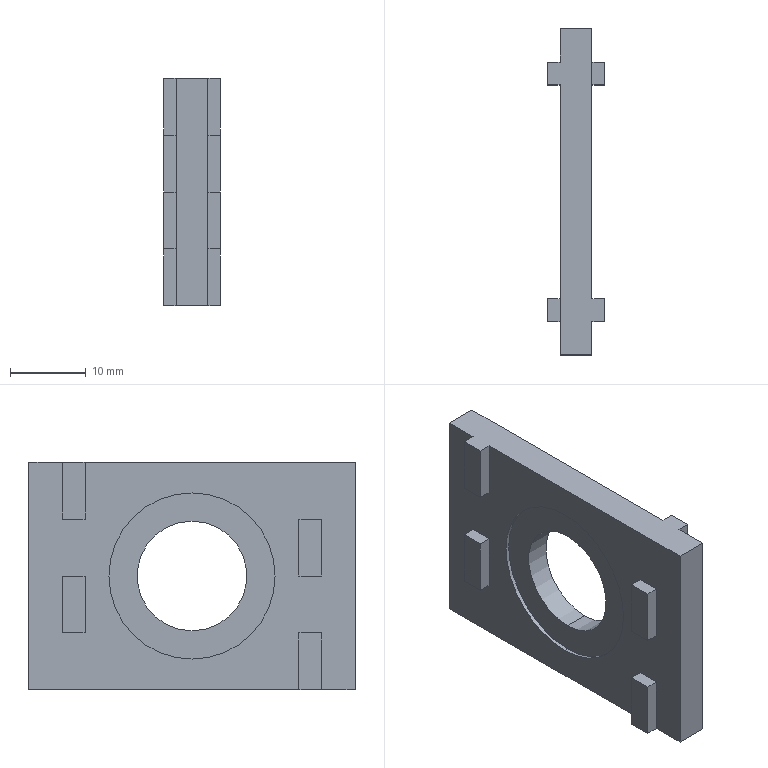Part | SolidWorks | features BaseBody 1 | 1 solid | 50 faces | box 7.5 x 43 x 30 mm | volume 4813 mm3 | plane 44 | cylinder 6 | commonest cylinder face diameters 21.9 x4 14.46 x2
STEP:
#1=CARTESIAN_POINT('',(-1.6,0.,7.23));
#2=VERTEX_POINT('',#1);
#3=CARTESIAN_POINT('',(-1.6,0.,-7.23));
#4=VERTEX_POINT('',#3);
#5=CARTESIAN_POINT('',(-1.6,0.,0.));
#6=DIRECTION('',(1.,0.,0.));
#7=DIRECTION('',(0.,0.,-1.));
#8=AXIS2_PLACEMENT_3D('',#5,#6,#7);
#9=CIRCLE('',#8,7.23);
#10=EDGE_CURVE('',#2,#4,#9,.T.);
#11=ORIENTED_EDGE('',*,*,#10,.F.);
#12=CARTESIAN_POINT('',(1.6,0.,7.23));
#13=VERTEX_POINT('',#12);
#14=CARTESIAN_POINT('',(2.1,0.,7.23));
#15=DIRECTION('',(1.,0.,0.));
#16=VECTOR('',#15,1000.);
#17=LINE('',#14,#16);
#18=EDGE_CURVE('',#2,#13,#17,.T.);
#19=ORIENTED_EDGE('',*,*,#18,.T.);
#20=CARTESIAN_POINT('',(1.6,0.,-7.23));
#21=VERTEX_POINT('',#20);
#22=CARTESIAN_POINT('',(1.6,0.,0.));
#23=DIRECTION('',(1.,0.,0.));
#24=DIRECTION('',(0.,0.,-1.));
#25=AXIS2_PLACEMENT_3D('',#22,#23,#24);
#26=CIRCLE('',#25,7.23);
#27=EDGE_CURVE('',#13,#21,#26,.T.);
#28=ORIENTED_EDGE('',*,*,#27,.T.);
#29=CARTESIAN_POINT('',(2.1,0.,-7.23));
#30=DIRECTION('',(1.,0.,0.));
#31=VECTOR('',#30,1000.);
#32=LINE('',#29,#31);
#33=EDGE_CURVE('',#4,#21,#32,.T.);
#34=ORIENTED_EDGE('',*,*,#33,.F.);
#35=EDGE_LOOP('',(#11,#19,#28,#34));
#36=FACE_OUTER_BOUND('',#35,.T.);
#37=CARTESIAN_POINT('',(2.1,0.,0.));
#38=DIRECTION('',(1.,0.,0.));
#39=DIRECTION('',(0.,0.,-1.));
#40=AXIS2_PLACEMENT_3D('',#37,#38,#39);
#41=CYLINDRICAL_SURFACE('',#40,7.23);
#42=ADVANCED_FACE('',(#36),#41,.F.);
#43=CARTESIAN_POINT('',(1.6,0.,10.95));
#44=VERTEX_POINT('',#43);
#45=CARTESIAN_POINT('',(1.6,0.,-10.95));
#46=VERTEX_POINT('',#45);
#47=CARTESIAN_POINT('',(1.6,0.,0.));
#48=DIRECTION('',(1.,0.,0.));
#49=DIRECTION('',(0.,0.,-1.));
#50=AXIS2_PLACEMENT_3D('',#47,#48,#49);
#51=CIRCLE('',#50,10.95);
#52=EDGE_CURVE('',#44,#46,#51,.T.);
#53=ORIENTED_EDGE('',*,*,#52,.F.);
#54=CARTESIAN_POINT('',(2.1,0.,10.95));
#55=VERTEX_POINT('',#54);
#56=CARTESIAN_POINT('',(2.1,0.,10.95));
#57=DIRECTION('',(1.,0.,0.));
#58=VECTOR('',#57,1000.);
#59=LINE('',#56,#58);
#60=EDGE_CURVE('',#44,#55,#59,.T.);
#61=ORIENTED_EDGE('',*,*,#60,.T.);
#62=CARTESIAN_POINT('',(2.1,0.,-10.95));
#63=VERTEX_POINT('',#62);
#64=CARTESIAN_POINT('',(2.1,0.,0.));
#65=DIRECTION('',(1.,0.,0.));
#66=DIRECTION('',(0.,0.,-1.));
#67=AXIS2_PLACEMENT_3D('',#64,#65,#66);
#68=CIRCLE('',#67,10.95);
#69=EDGE_CURVE('',#55,#63,#68,.T.);
#70=ORIENTED_EDGE('',*,*,#69,.T.);
#71=CARTESIAN_POINT('',(2.1,0.,-10.95));
#72=DIRECTION('',(1.,0.,0.));
#73=VECTOR('',#72,1000.);
#74=LINE('',#71,#73);
#75=EDGE_CURVE('',#46,#63,#74,.T.);
#76=ORIENTED_EDGE('',*,*,#75,.F.);
#77=EDGE_LOOP('',(#53,#61,#70,#76));
#78=FACE_OUTER_BOUND('',#77,.T.);
#79=CARTESIAN_POINT('',(2.1,0.,0.));
#80=DIRECTION('',(1.,0.,0.));
#81=DIRECTION('',(0.,0.,-1.));
#82=AXIS2_PLACEMENT_3D('',#79,#80,#81);
#83=CYLINDRICAL_SURFACE('',#82,10.95);
#84=ADVANCED_FACE('',(#78),#83,.F.);
#85=CARTESIAN_POINT('',(-2.1,0.,10.95));
#86=VERTEX_POINT('',#85);
#87=CARTESIAN_POINT('',(-2.1,0.,-10.95));
#88=VERTEX_POINT('',#87);
#89=CARTESIAN_POINT('',(-2.1,0.,0.));
#90=DIRECTION('',(1.,0.,0.));
#91=DIRECTION('',(0.,0.,-1.));
#92=AXIS2_PLACEMENT_3D('',#89,#90,#91);
#93=CIRCLE('',#92,10.95);
#94=EDGE_CURVE('',#86,#88,#93,.T.);
#95=ORIENTED_EDGE('',*,*,#94,.F.);
#96=CARTESIAN_POINT('',(-1.6,0.,10.95));
#97=VERTEX_POINT('',#96);
#98=CARTESIAN_POINT('',(2.1,0.,10.95));
#99=DIRECTION('',(1.,0.,0.));
#100=VECTOR('',#99,1000.);
#101=LINE('',#98,#100);
#102=EDGE_CURVE('',#86,#97,#101,.T.);
#103=ORIENTED_EDGE('',*,*,#102,.T.);
#104=CARTESIAN_POINT('',(-1.6,0.,-10.95));
#105=VERTEX_POINT('',#104);
#106=CARTESIAN_POINT('',(-1.6,0.,0.));
#107=DIRECTION('',(1.,0.,0.));
#108=DIRECTION('',(0.,0.,-1.));
#109=AXIS2_PLACEMENT_3D('',#106,#107,#108);
#110=CIRCLE('',#109,10.95);
#111=EDGE_CURVE('',#97,#105,#110,.T.);
#112=ORIENTED_EDGE('',*,*,#111,.T.);
#113=CARTESIAN_POINT('',(2.1,0.,-10.95));
#114=DIRECTION('',(1.,0.,0.));
#115=VECTOR('',#114,1000.);
#116=LINE('',#113,#115);
#117=EDGE_CURVE('',#88,#105,#116,.T.);
#118=ORIENTED_EDGE('',*,*,#117,.F.);
#119=EDGE_LOOP('',(#95,#103,#112,#118));
#120=FACE_OUTER_BOUND('',#119,.T.);
#121=CARTESIAN_POINT('',(2.1,0.,0.));
#122=DIRECTION('',(1.,0.,0.));
#123=DIRECTION('',(0.,0.,-1.));
#124=AXIS2_PLACEMENT_3D('',#121,#122,#123);
#125=CYLINDRICAL_SURFACE('',#124,10.95);
#126=ADVANCED_FACE('',(#120),#125,.F.);
#127=CARTESIAN_POINT('',(-3.75,-14.1,-7.5));
#128=VERTEX_POINT('',#127);
#129=CARTESIAN_POINT('',(-3.75,-14.1,-15.));
#130=VERTEX_POINT('',#129);
#131=CARTESIAN_POINT('',(-3.75,-14.1,-7.5));
#132=DIRECTION('',(0.,0.,-1.));
#133=VECTOR('',#132,1000.);
#134=LINE('',#131,#133);
#135=EDGE_CURVE('',#128,#130,#134,.T.);
#136=ORIENTED_EDGE('',*,*,#135,.F.);
#137=CARTESIAN_POINT('',(-2.1,-14.1,-7.5));
#138=VERTEX_POINT('',#137);
#139=CARTESIAN_POINT('',(-3.75,-14.1,-7.5));
#140=DIRECTION('',(1.,0.,0.));
#141=VECTOR('',#140,1000.);
#142=LINE('',#139,#141);
#143=EDGE_CURVE('',#128,#138,#142,.T.);
#144=ORIENTED_EDGE('',*,*,#143,.T.);
#145=CARTESIAN_POINT('',(-2.1,-14.1,-15.));
#146=VERTEX_POINT('',#145);
#147=CARTESIAN_POINT('',(-2.1,-14.1,-7.5));
#148=DIRECTION('',(0.,0.,-1.));
#149=VECTOR('',#148,1000.);
#150=LINE('',#147,#149);
#151=EDGE_CURVE('',#138,#146,#150,.T.);
#152=ORIENTED_EDGE('',*,*,#151,.T.);
#153=CARTESIAN_POINT('',(-2.1,-14.1,-15.));
#154=DIRECTION('',(-1.,0.,0.));
#155=VECTOR('',#154,1000.);
#156=LINE('',#153,#155);
#157=EDGE_CURVE('',#146,#130,#156,.T.);
#158=ORIENTED_EDGE('',*,*,#157,.T.);
#159=EDGE_LOOP('',(#136,#144,#152,#158));
#160=FACE_OUTER_BOUND('',#159,.T.);
#161=CARTESIAN_POINT('',(-2.1,-14.1,15.));
#162=DIRECTION('',(0.,-1.,0.));
#163=DIRECTION('',(0.,0.,-1.));
#164=AXIS2_PLACEMENT_3D('',#161,#162,#163);
#165=PLANE('',#164);
#166=ADVANCED_FACE('',(#160),#165,.F.);
#167=CARTESIAN_POINT('',(-3.75,-17.1,-7.5));
#168=VERTEX_POINT('',#167);
#169=CARTESIAN_POINT('',(-3.75,-17.1,-15.));
#170=VERTEX_POINT('',#169);
#171=CARTESIAN_POINT('',(-3.75,-17.1,-7.5));
#172=DIRECTION('',(0.,0.,-1.));
#173=VECTOR('',#172,1000.);
#174=LINE('',#171,#173);
#175=EDGE_CURVE('',#168,#170,#174,.T.);
#176=ORIENTED_EDGE('',*,*,#175,.F.);
#177=CARTESIAN_POINT('',(-3.75,-17.1,-7.5));
#178=DIRECTION('',(0.,1.,0.));
#179=VECTOR('',#178,1000.);
#180=LINE('',#177,#179);
#181=EDGE_CURVE('',#168,#128,#180,.T.);
#182=ORIENTED_EDGE('',*,*,#181,.T.);
#183=ORIENTED_EDGE('',*,*,#135,.T.);
#184=CARTESIAN_POINT('',(-3.75,-14.1,-15.));
#185=DIRECTION('',(0.,-1.,0.));
#186=VECTOR('',#185,1000.);
#187=LINE('',#184,#186);
#188=EDGE_CURVE('',#130,#170,#187,.T.);
#189=ORIENTED_EDGE('',*,*,#188,.T.);
#190=EDGE_LOOP('',(#176,#182,#183,#189));
#191=FACE_OUTER_BOUND('',#190,.T.);
#192=CARTESIAN_POINT('',(-3.75,-14.1,15.));
#193=DIRECTION('',(1.,0.,0.));
#194=DIRECTION('',(0.,0.,-1.));
#195=AXIS2_PLACEMENT_3D('',#192,#193,#194);
#196=PLANE('',#195);
#197=ADVANCED_FACE('',(#191),#196,.F.);
#198=ORIENTED_EDGE('',*,*,#181,.F.);
#199=CARTESIAN_POINT('',(-2.1,-17.1,-7.5));
#200=VERTEX_POINT('',#199);
#201=CARTESIAN_POINT('',(-2.1,-17.1,-7.5));
#202=DIRECTION('',(-1.,0.,0.));
#203=VECTOR('',#202,1000.);
#204=LINE('',#201,#203);
#205=EDGE_CURVE('',#200,#168,#204,.T.);
#206=ORIENTED_EDGE('',*,*,#205,.F.);
#207=CARTESIAN_POINT('',(-2.1,-17.1,-7.5));
#208=DIRECTION('',(0.,1.,0.));
#209=VECTOR('',#208,1000.);
#210=LINE('',#207,#209);
#211=EDGE_CURVE('',#200,#138,#210,.T.);
#212=ORIENTED_EDGE('',*,*,#211,.T.);
#213=ORIENTED_EDGE('',*,*,#143,.F.);
#214=EDGE_LOOP('',(#198,#206,#212,#213));
#215=FACE_OUTER_BOUND('',#214,.T.);
#216=CARTESIAN_POINT('',(-2.1,-21.5,-7.5));
#217=DIRECTION('',(0.,0.,-1.));
#218=DIRECTION('',(-1.,0.,0.));
#219=AXIS2_PLACEMENT_3D('',#216,#217,#218);
#220=PLANE('',#219);
#221=ADVANCED_FACE('',(#215),#220,.F.);
#222=CARTESIAN_POINT('',(-2.1,0.,0.));
#223=DIRECTION('',(1.,0.,0.));
#224=DIRECTION('',(0.,0.,-1.));
#225=AXIS2_PLACEMENT_3D('',#222,#223,#224);
#226=CIRCLE('',#225,10.95);
#227=EDGE_CURVE('',#88,#86,#226,.T.);
#228=ORIENTED_EDGE('',*,*,#227,.T.);
#229=ORIENTED_EDGE('',*,*,#94,.T.);
#230=EDGE_LOOP('',(#228,#229));
#231=FACE_BOUND('',#230,.T.);
#232=CARTESIAN_POINT('',(-2.1,-14.1,7.5));
#233=VERTEX_POINT('',#232);
#234=CARTESIAN_POINT('',(-2.1,-14.1,0.));
#235=VERTEX_POINT('',#234);
#236=CARTESIAN_POINT('',(-2.1,-14.1,7.5));
#237=DIRECTION('',(0.,0.,-1.));
#238=VECTOR('',#237,1000.);
#239=LINE('',#236,#238);
#240=EDGE_CURVE('',#233,#235,#239,.T.);
#241=ORIENTED_EDGE('',*,*,#240,.F.);
#242=CARTESIAN_POINT('',(-2.1,-17.1,7.5));
#243=VERTEX_POINT('',#242);
#244=CARTESIAN_POINT('',(-2.1,-17.1,7.5));
#245=DIRECTION('',(0.,1.,0.));
#246=VECTOR('',#245,1000.);
#247=LINE('',#244,#246);
#248=EDGE_CURVE('',#243,#233,#247,.T.);
#249=ORIENTED_EDGE('',*,*,#248,.F.);
#250=CARTESIAN_POINT('',(-2.1,-17.1,0.));
#251=VERTEX_POINT('',#250);
#252=CARTESIAN_POINT('',(-2.1,-17.1,7.5));
#253=DIRECTION('',(0.,0.,-1.));
#254=VECTOR('',#253,1000.);
#255=LINE('',#252,#254);
#256=EDGE_CURVE('',#243,#251,#255,.T.);
#257=ORIENTED_EDGE('',*,*,#256,.T.);
#258=CARTESIAN_POINT('',(-2.1,-17.1,0.));
#259=DIRECTION('',(0.,1.,0.));
#260=VECTOR('',#259,1000.);
#261=LINE('',#258,#260);
#262=EDGE_CURVE('',#251,#235,#261,.T.);
#263=ORIENTED_EDGE('',*,*,#262,.T.);
#264=EDGE_LOOP('',(#241,#249,#257,#263));
#265=FACE_BOUND('',#264,.T.);
#266=ORIENTED_EDGE('',*,*,#151,.F.);
#267=ORIENTED_EDGE('',*,*,#211,.F.);
#268=CARTESIAN_POINT('',(-2.1,-17.1,-15.));
#269=VERTEX_POINT('',#268);
#270=CARTESIAN_POINT('',(-2.1,-17.1,-7.5));
#271=DIRECTION('',(0.,0.,-1.));
#272=VECTOR('',#271,1000.);
#273=LINE('',#270,#272);
#274=EDGE_CURVE('',#200,#269,#273,.T.);
#275=ORIENTED_EDGE('',*,*,#274,.T.);
#276=CARTESIAN_POINT('',(-2.1,-21.5,-15.));
#277=VERTEX_POINT('',#276);
#278=CARTESIAN_POINT('',(-2.1,-17.1,-15.));
#279=DIRECTION('',(0.,-1.,0.));
#280=VECTOR('',#279,1000.);
#281=LINE('',#278,#280);
#282=EDGE_CURVE('',#269,#277,#281,.T.);
#283=ORIENTED_EDGE('',*,*,#282,.T.);
#284=CARTESIAN_POINT('',(-2.1,-21.5,15.));
#285=VERTEX_POINT('',#284);
#286=CARTESIAN_POINT('',(-2.1,-21.5,15.));
#287=DIRECTION('',(0.,0.,-1.));
#288=VECTOR('',#287,1000.);
#289=LINE('',#286,#288);
#290=EDGE_CURVE('',#285,#277,#289,.T.);
#291=ORIENTED_EDGE('',*,*,#290,.F.);
#292=CARTESIAN_POINT('',(-2.1,14.1,15.));
#293=VERTEX_POINT('',#292);
#294=CARTESIAN_POINT('',(-2.1,14.1,15.));
#295=DIRECTION('',(0.,-1.,0.));
#296=VECTOR('',#295,1000.);
#297=LINE('',#294,#296);
#298=EDGE_CURVE('',#293,#285,#297,.T.);
#299=ORIENTED_EDGE('',*,*,#298,.F.);
#300=CARTESIAN_POINT('',(-2.1,14.1,7.5));
#301=VERTEX_POINT('',#300);
#302=CARTESIAN_POINT('',(-2.1,14.1,15.));
#303=DIRECTION('',(0.,0.,-1.));
#304=VECTOR('',#303,1000.);
#305=LINE('',#302,#304);
#306=EDGE_CURVE('',#293,#301,#305,.T.);
#307=ORIENTED_EDGE('',*,*,#306,.T.);
#308=CARTESIAN_POINT('',(-2.1,17.1,7.5));
#309=VERTEX_POINT('',#308);
#310=CARTESIAN_POINT('',(-2.1,17.1,7.5));
#311=DIRECTION('',(0.,-1.,0.));
#312=VECTOR('',#311,1000.);
#313=LINE('',#310,#312);
#314=EDGE_CURVE('',#309,#301,#313,.T.);
#315=ORIENTED_EDGE('',*,*,#314,.F.);
#316=CARTESIAN_POINT('',(-2.1,17.1,15.));
#317=VERTEX_POINT('',#316);
#318=CARTESIAN_POINT('',(-2.1,17.1,15.));
#319=DIRECTION('',(0.,0.,-1.));
#320=VECTOR('',#319,1000.);
#321=LINE('',#318,#320);
#322=EDGE_CURVE('',#317,#309,#321,.T.);
#323=ORIENTED_EDGE('',*,*,#322,.F.);
#324=CARTESIAN_POINT('',(-2.1,21.5,15.));
#325=VERTEX_POINT('',#324);
#326=CARTESIAN_POINT('',(-2.1,21.5,15.));
#327=DIRECTION('',(0.,-1.,0.));
#328=VECTOR('',#327,1000.);
#329=LINE('',#326,#328);
#330=EDGE_CURVE('',#325,#317,#329,.T.);
#331=ORIENTED_EDGE('',*,*,#330,.F.);
#332=CARTESIAN_POINT('',(-2.1,21.5,-15.));
#333=VERTEX_POINT('',#332);
#334=CARTESIAN_POINT('',(-2.1,21.5,15.));
#335=DIRECTION('',(0.,0.,-1.));
#336=VECTOR('',#335,1000.);
#337=LINE('',#334,#336);
#338=EDGE_CURVE('',#325,#333,#337,.T.);
#339=ORIENTED_EDGE('',*,*,#338,.T.);
#340=CARTESIAN_POINT('',(-2.1,21.5,-15.));
#341=DIRECTION('',(0.,-1.,0.));
#342=VECTOR('',#341,1000.);
#343=LINE('',#340,#342);
#344=EDGE_CURVE('',#333,#146,#343,.T.);
#345=ORIENTED_EDGE('',*,*,#344,.T.);
#346=EDGE_LOOP('',(#266,#267,#275,#283,#291,#299,#307,#315,#323,#331,#339,#345));
#347=FACE_OUTER_BOUND('',#346,.T.);
#348=CARTESIAN_POINT('',(-2.1,17.1,0.));
#349=VERTEX_POINT('',#348);
#350=CARTESIAN_POINT('',(-2.1,14.1,0.));
#351=VERTEX_POINT('',#350);
#352=CARTESIAN_POINT('',(-2.1,17.1,0.));
#353=DIRECTION('',(0.,-1.,0.));
#354=VECTOR('',#353,1000.);
#355=LINE('',#352,#354);
#356=EDGE_CURVE('',#349,#351,#355,.T.);
#357=ORIENTED_EDGE('',*,*,#356,.T.);
#358=CARTESIAN_POINT('',(-2.1,14.1,-7.5));
#359=VERTEX_POINT('',#358);
#360=CARTESIAN_POINT('',(-2.1,14.1,0.));
#361=DIRECTION('',(0.,0.,-1.));
#362=VECTOR('',#361,1000.);
#363=LINE('',#360,#362);
#364=EDGE_CURVE('',#351,#359,#363,.T.);
#365=ORIENTED_EDGE('',*,*,#364,.T.);
#366=CARTESIAN_POINT('',(-2.1,17.1,-7.5));
#367=VERTEX_POINT('',#366);
#368=CARTESIAN_POINT('',(-2.1,17.1,-7.5));
#369=DIRECTION('',(0.,-1.,0.));
#370=VECTOR('',#369,1000.);
#371=LINE('',#368,#370);
#372=EDGE_CURVE('',#367,#359,#371,.T.);
#373=ORIENTED_EDGE('',*,*,#372,.F.);
#374=CARTESIAN_POINT('',(-2.1,17.1,0.));
#375=DIRECTION('',(0.,0.,-1.));
#376=VECTOR('',#375,1000.);
#377=LINE('',#374,#376);
#378=EDGE_CURVE('',#349,#367,#377,.T.);
#379=ORIENTED_EDGE('',*,*,#378,.F.);
#380=EDGE_LOOP('',(#357,#365,#373,#379));
#381=FACE_BOUND('',#380,.T.);
#382=CARTESIAN_POINT('',(-2.1,21.5,15.));
#383=DIRECTION('',(1.,0.,0.));
#384=DIRECTION('',(0.,0.,-1.));
#385=AXIS2_PLACEMENT_3D('',#382,#383,#384);
#386=PLANE('',#385);
#387=ADVANCED_FACE('',(#231,#265,#347,#381),#386,.F.);
#388=ORIENTED_EDGE('',*,*,#157,.F.);
#389=ORIENTED_EDGE('',*,*,#344,.F.);
#390=CARTESIAN_POINT('',(2.1,21.5,-15.));
#391=VERTEX_POINT('',#390);
#392=CARTESIAN_POINT('',(2.1,21.5,-15.));
#393=DIRECTION('',(-1.,0.,0.));
#394=VECTOR('',#393,1000.);
#395=LINE('',#392,#394);
#396=EDGE_CURVE('',#391,#333,#395,.T.);
#397=ORIENTED_EDGE('',*,*,#396,.F.);
#398=CARTESIAN_POINT('',(2.1,17.1,-15.));
#399=VERTEX_POINT('',#398);
#400=CARTESIAN_POINT('',(2.1,17.1,-15.));
#401=DIRECTION('',(0.,1.,0.));
#402=VECTOR('',#401,1000.);
#403=LINE('',#400,#402);
#404=EDGE_CURVE('',#399,#391,#403,.T.);
#405=ORIENTED_EDGE('',*,*,#404,.F.);
#406=CARTESIAN_POINT('',(3.75,17.1,-15.));
#407=VERTEX_POINT('',#406);
#408=CARTESIAN_POINT('',(3.75,17.1,-15.));
#409=DIRECTION('',(-1.,0.,0.));
#410=VECTOR('',#409,1000.);
#411=LINE('',#408,#410);
#412=EDGE_CURVE('',#407,#399,#411,.T.);
#413=ORIENTED_EDGE('',*,*,#412,.F.);
#414=CARTESIAN_POINT('',(3.75,14.1,-15.));
#415=VERTEX_POINT('',#414);
#416=CARTESIAN_POINT('',(3.75,14.1,-15.));
#417=DIRECTION('',(0.,1.,0.));
#418=VECTOR('',#417,1000.);
#419=LINE('',#416,#418);
#420=EDGE_CURVE('',#415,#407,#419,.T.);
#421=ORIENTED_EDGE('',*,*,#420,.F.);
#422=CARTESIAN_POINT('',(2.1,14.1,-15.));
#423=VERTEX_POINT('',#422);
#424=CARTESIAN_POINT('',(2.1,14.1,-15.));
#425=DIRECTION('',(1.,0.,0.));
#426=VECTOR('',#425,1000.);
#427=LINE('',#424,#426);
#428=EDGE_CURVE('',#423,#415,#427,.T.);
#429=ORIENTED_EDGE('',*,*,#428,.F.);
#430=CARTESIAN_POINT('',(2.1,-21.5,-15.));
#431=VERTEX_POINT('',#430);
#432=CARTESIAN_POINT('',(2.1,-21.5,-15.));
#433=DIRECTION('',(0.,1.,0.));
#434=VECTOR('',#433,1000.);
#435=LINE('',#432,#434);
#436=EDGE_CURVE('',#431,#423,#435,.T.);
#437=ORIENTED_EDGE('',*,*,#436,.F.);
#438=CARTESIAN_POINT('',(-2.1,-21.5,-15.));
#439=DIRECTION('',(1.,0.,0.));
#440=VECTOR('',#439,1000.);
#441=LINE('',#438,#440);
#442=EDGE_CURVE('',#277,#431,#441,.T.);
#443=ORIENTED_EDGE('',*,*,#442,.F.);
#444=ORIENTED_EDGE('',*,*,#282,.F.);
#445=CARTESIAN_POINT('',(-3.75,-17.1,-15.));
#446=DIRECTION('',(1.,0.,0.));
#447=VECTOR('',#446,1000.);
#448=LINE('',#445,#447);
#449=EDGE_CURVE('',#170,#269,#448,.T.);
#450=ORIENTED_EDGE('',*,*,#449,.F.);
#451=ORIENTED_EDGE('',*,*,#188,.F.);
#452=EDGE_LOOP('',(#388,#389,#397,#405,#413,#421,#429,#437,#443,#444,#450,#451));
#453=FACE_OUTER_BOUND('',#452,.T.);
#454=CARTESIAN_POINT('',(0.,0.,-15.));
#455=DIRECTION('',(0.,0.,1.));
#456=DIRECTION('',(1.,0.,0.));
#457=AXIS2_PLACEMENT_3D('',#454,#455,#456);
#458=PLANE('',#457);
#459=ADVANCED_FACE('',(#453),#458,.F.);
#460=ORIENTED_EDGE('',*,*,#274,.F.);
#461=ORIENTED_EDGE('',*,*,#205,.T.);
#462=ORIENTED_EDGE('',*,*,#175,.T.);
#463=ORIENTED_EDGE('',*,*,#449,.T.);
#464=EDGE_LOOP('',(#460,#461,#462,#463));
#465=FACE_OUTER_BOUND('',#464,.T.);
#466=CARTESIAN_POINT('',(-3.75,-17.1,15.));
#467=DIRECTION('',(0.,1.,0.));
#468=DIRECTION('',(0.,0.,1.));
#469=AXIS2_PLACEMENT_3D('',#466,#467,#468);
#470=PLANE('',#469);
#471=ADVANCED_FACE('',(#465),#470,.F.);
#472=ORIENTED_EDGE('',*,*,#102,.F.);
#473=ORIENTED_EDGE('',*,*,#227,.F.);
#474=ORIENTED_EDGE('',*,*,#117,.T.);
#475=CARTESIAN_POINT('',(-1.6,0.,0.));
#476=DIRECTION('',(1.,0.,0.));
#477=DIRECTION('',(0.,0.,-1.));
#478=AXIS2_PLACEMENT_3D('',#475,#476,#477);
#479=CIRCLE('',#478,10.95);
#480=EDGE_CURVE('',#105,#97,#479,.T.);
#481=ORIENTED_EDGE('',*,*,#480,.T.);
#482=EDGE_LOOP('',(#472,#473,#474,#481));
#483=FACE_OUTER_BOUND('',#482,.T.);
#484=CARTESIAN_POINT('',(2.1,0.,0.));
#485=DIRECTION('',(1.,0.,0.));
#486=DIRECTION('',(0.,0.,-1.));
#487=AXIS2_PLACEMENT_3D('',#484,#485,#486);
#488=CYLINDRICAL_SURFACE('',#487,10.95);
#489=ADVANCED_FACE('',(#483),#488,.F.);
#490=CARTESIAN_POINT('',(-3.75,-14.1,7.5));
#491=VERTEX_POINT('',#490);
#492=CARTESIAN_POINT('',(-3.75,-14.1,0.));
#493=VERTEX_POINT('',#492);
#494=CARTESIAN_POINT('',(-3.75,-14.1,7.5));
#495=DIRECTION('',(0.,0.,-1.));
#496=VECTOR('',#495,1000.);
#497=LINE('',#494,#496);
#498=EDGE_CURVE('',#491,#493,#497,.T.);
#499=ORIENTED_EDGE('',*,*,#498,.F.);
#500=CARTESIAN_POINT('',(-3.75,-14.1,7.5));
#501=DIRECTION('',(1.,0.,0.));
#502=VECTOR('',#501,1000.);
#503=LINE('',#500,#502);
#504=EDGE_CURVE('',#491,#233,#503,.T.);
#505=ORIENTED_EDGE('',*,*,#504,.T.);
#506=ORIENTED_EDGE('',*,*,#240,.T.);
#507=CARTESIAN_POINT('',(-2.1,-14.1,0.));
#508=DIRECTION('',(-1.,0.,0.));
#509=VECTOR('',#508,1000.);
#510=LINE('',#507,#509);
#511=EDGE_CURVE('',#235,#493,#510,.T.);
#512=ORIENTED_EDGE('',*,*,#511,.T.);
#513=EDGE_LOOP('',(#499,#505,#506,#512));
#514=FACE_OUTER_BOUND('',#513,.T.);
#515=CARTESIAN_POINT('',(-2.1,-14.1,15.));
#516=DIRECTION('',(0.,-1.,0.));
#517=DIRECTION('',(0.,0.,-1.));
#518=AXIS2_PLACEMENT_3D('',#515,#516,#517);
#519=PLANE('',#518);
#520=ADVANCED_FACE('',(#514),#519,.F.);
#521=CARTESIAN_POINT('',(-3.75,-17.1,7.5));
#522=VERTEX_POINT('',#521);
#523=CARTESIAN_POINT('',(-3.75,-17.1,7.5));
#524=DIRECTION('',(0.,1.,0.));
#525=VECTOR('',#524,1000.);
#526=LINE('',#523,#525);
#527=EDGE_CURVE('',#522,#491,#526,.T.);
#528=ORIENTED_EDGE('',*,*,#527,.F.);
#529=CARTESIAN_POINT('',(-2.1,-17.1,7.5));
#530=DIRECTION('',(-1.,0.,0.));
#531=VECTOR('',#530,1000.);
#532=LINE('',#529,#531);
#533=EDGE_CURVE('',#243,#522,#532,.T.);
#534=ORIENTED_EDGE('',*,*,#533,.F.);
#535=ORIENTED_EDGE('',*,*,#248,.T.);
#536=ORIENTED_EDGE('',*,*,#504,.F.);
#537=EDGE_LOOP('',(#528,#534,#535,#536));
#538=FACE_OUTER_BOUND('',#537,.T.);
#539=CARTESIAN_POINT('',(-2.1,-21.5,7.5));
#540=DIRECTION('',(0.,0.,-1.));
#541=DIRECTION('',(-1.,0.,0.));
#542=AXIS2_PLACEMENT_3D('',#539,#540,#541);
#543=PLANE('',#542);
#544=ADVANCED_FACE('',(#538),#543,.F.);
#545=ORIENTED_EDGE('',*,*,#256,.F.);
#546=ORIENTED_EDGE('',*,*,#533,.T.);
#547=CARTESIAN_POINT('',(-3.75,-17.1,0.));
#548=VERTEX_POINT('',#547);
#549=CARTESIAN_POINT('',(-3.75,-17.1,7.5));
#550=DIRECTION('',(0.,0.,-1.));
#551=VECTOR('',#550,1000.);
#552=LINE('',#549,#551);
#553=EDGE_CURVE('',#522,#548,#552,.T.);
#554=ORIENTED_EDGE('',*,*,#553,.T.);
#555=CARTESIAN_POINT('',(-3.75,-17.1,0.));
#556=DIRECTION('',(1.,0.,0.));
#557=VECTOR('',#556,1000.);
#558=LINE('',#555,#557);
#559=EDGE_CURVE('',#548,#251,#558,.T.);
#560=ORIENTED_EDGE('',*,*,#559,.T.);
#561=EDGE_LOOP('',(#545,#546,#554,#560));
#562=FACE_OUTER_BOUND('',#561,.T.);
#563=CARTESIAN_POINT('',(-3.75,-17.1,15.));
#564=DIRECTION('',(0.,1.,0.));
#565=DIRECTION('',(0.,0.,1.));
#566=AXIS2_PLACEMENT_3D('',#563,#564,#565);
#567=PLANE('',#566);
#568=ADVANCED_FACE('',(#562),#567,.F.);
#569=ORIENTED_EDGE('',*,*,#262,.F.);
#570=ORIENTED_EDGE('',*,*,#559,.F.);
#571=CARTESIAN_POINT('',(-3.75,-17.1,0.));
#572=DIRECTION('',(0.,1.,0.));
#573=VECTOR('',#572,1000.);
#574=LINE('',#571,#573);
#575=EDGE_CURVE('',#548,#493,#574,.T.);
#576=ORIENTED_EDGE('',*,*,#575,.T.);
#577=ORIENTED_EDGE('',*,*,#511,.F.);
#578=EDGE_LOOP('',(#569,#570,#576,#577));
#579=FACE_OUTER_BOUND('',#578,.T.);
#580=CARTESIAN_POINT('',(-3.75,-21.5,0.));
#581=DIRECTION('',(0.,0.,1.));
#582=DIRECTION('',(1.,0.,0.));
#583=AXIS2_PLACEMENT_3D('',#580,#581,#582);
#584=PLANE('',#583);
#585=ADVANCED_FACE('',(#579),#584,.F.);
#586=ORIENTED_EDGE('',*,*,#442,.T.);
#587=CARTESIAN_POINT('',(2.1,-21.5,15.));
#588=VERTEX_POINT('',#587);
#589=CARTESIAN_POINT('',(2.1,-21.5,15.));
#590=DIRECTION('',(0.,0.,-1.));
#591=VECTOR('',#590,1000.);
#592=LINE('',#589,#591);
#593=EDGE_CURVE('',#588,#431,#592,.T.);
#594=ORIENTED_EDGE('',*,*,#593,.F.);
#595=CARTESIAN_POINT('',(-2.1,-21.5,15.));
#596=DIRECTION('',(1.,0.,0.));
#597=VECTOR('',#596,1000.);
#598=LINE('',#595,#597);
#599=EDGE_CURVE('',#285,#588,#598,.T.);
#600=ORIENTED_EDGE('',*,*,#599,.F.);
#601=ORIENTED_EDGE('',*,*,#290,.T.);
#602=EDGE_LOOP('',(#586,#594,#600,#601));
#603=FACE_OUTER_BOUND('',#602,.T.);
#604=CARTESIAN_POINT('',(-2.1,-21.5,15.));
#605=DIRECTION('',(0.,1.,0.));
#606=DIRECTION('',(0.,0.,1.));
#607=AXIS2_PLACEMENT_3D('',#604,#605,#606);
#608=PLANE('',#607);
#609=ADVANCED_FACE('',(#603),#608,.F.);
#610=ORIENTED_EDGE('',*,*,#298,.T.);
#611=ORIENTED_EDGE('',*,*,#599,.T.);
#612=CARTESIAN_POINT('',(2.1,-17.1,15.));
#613=VERTEX_POINT('',#612);
#614=CARTESIAN_POINT('',(2.1,-21.5,15.));
#615=DIRECTION('',(0.,1.,0.));
#616=VECTOR('',#615,1000.);
#617=LINE('',#614,#616);
#618=EDGE_CURVE('',#588,#613,#617,.T.);
#619=ORIENTED_EDGE('',*,*,#618,.T.);
#620=CARTESIAN_POINT('',(3.75,-17.1,15.));
#621=VERTEX_POINT('',#620);
#622=CARTESIAN_POINT('',(2.1,-17.1,15.));
#623=DIRECTION('',(1.,0.,0.));
#624=VECTOR('',#623,1000.);
#625=LINE('',#622,#624);
#626=EDGE_CURVE('',#613,#621,#625,.T.);
#627=ORIENTED_EDGE('',*,*,#626,.T.);
#628=CARTESIAN_POINT('',(3.75,-14.1,15.));
#629=VERTEX_POINT('',#628);
#630=CARTESIAN_POINT('',(3.75,-17.1,15.));
#631=DIRECTION('',(0.,1.,0.));
#632=VECTOR('',#631,1000.);
#633=LINE('',#630,#632);
#634=EDGE_CURVE('',#621,#629,#633,.T.);
#635=ORIENTED_EDGE('',*,*,#634,.T.);
#636=CARTESIAN_POINT('',(2.1,-14.1,15.));
#637=VERTEX_POINT('',#636);
#638=CARTESIAN_POINT('',(3.75,-14.1,15.));
#639=DIRECTION('',(-1.,0.,0.));
#640=VECTOR('',#639,1000.);
#641=LINE('',#638,#640);
#642=EDGE_CURVE('',#629,#637,#641,.T.);
#643=ORIENTED_EDGE('',*,*,#642,.T.);
#644=CARTESIAN_POINT('',(2.1,21.5,15.));
#645=VERTEX_POINT('',#644);
#646=CARTESIAN_POINT('',(2.1,-14.1,15.));
#647=DIRECTION('',(0.,1.,0.));
#648=VECTOR('',#647,1000.);
#649=LINE('',#646,#648);
#650=EDGE_CURVE('',#637,#645,#649,.T.);
#651=ORIENTED_EDGE('',*,*,#650,.T.);
#652=CARTESIAN_POINT('',(2.1,21.5,15.));
#653=DIRECTION('',(-1.,0.,0.));
#654=VECTOR('',#653,1000.);
#655=LINE('',#652,#654);
#656=EDGE_CURVE('',#645,#325,#655,.T.);
#657=ORIENTED_EDGE('',*,*,#656,.T.);
#658=ORIENTED_EDGE('',*,*,#330,.T.);
#659=CARTESIAN_POINT('',(-3.75,17.1,15.));
#660=VERTEX_POINT('',#659);
#661=CARTESIAN_POINT('',(-2.1,17.1,15.));
#662=DIRECTION('',(-1.,0.,0.));
#663=VECTOR('',#662,1000.);
#664=LINE('',#661,#663);
#665=EDGE_CURVE('',#317,#660,#664,.T.);
#666=ORIENTED_EDGE('',*,*,#665,.T.);
#667=CARTESIAN_POINT('',(-3.75,14.1,15.));
#668=VERTEX_POINT('',#667);
#669=CARTESIAN_POINT('',(-3.75,17.1,15.));
#670=DIRECTION('',(0.,-1.,0.));
#671=VECTOR('',#670,1000.);
#672=LINE('',#669,#671);
#673=EDGE_CURVE('',#660,#668,#672,.T.);
#674=ORIENTED_EDGE('',*,*,#673,.T.);
#675=CARTESIAN_POINT('',(-3.75,14.1,15.));
#676=DIRECTION('',(1.,0.,0.));
#677=VECTOR('',#676,1000.);
#678=LINE('',#675,#677);
#679=EDGE_CURVE('',#668,#293,#678,.T.);
#680=ORIENTED_EDGE('',*,*,#679,.T.);
#681=EDGE_LOOP('',(#610,#611,#619,#627,#635,#643,#651,#657,#658,#666,#674,#680));
#682=FACE_OUTER_BOUND('',#681,.T.);
#683=CARTESIAN_POINT('',(0.,0.,15.));
#684=DIRECTION('',(0.,0.,1.));
#685=DIRECTION('',(1.,0.,0.));
#686=AXIS2_PLACEMENT_3D('',#683,#684,#685);
#687=PLANE('',#686);
#688=ADVANCED_FACE('',(#682),#687,.T.);
#689=CARTESIAN_POINT('',(-3.75,14.1,7.5));
#690=VERTEX_POINT('',#689);
#691=CARTESIAN_POINT('',(-2.1,14.1,7.5));
#692=DIRECTION('',(-1.,0.,0.));
#693=VECTOR('',#692,1000.);
#694=LINE('',#691,#693);
#695=EDGE_CURVE('',#301,#690,#694,.T.);
#696=ORIENTED_EDGE('',*,*,#695,.F.);
#697=ORIENTED_EDGE('',*,*,#306,.F.);
#698=ORIENTED_EDGE('',*,*,#679,.F.);
#699=CARTESIAN_POINT('',(-3.75,14.1,15.));
#700=DIRECTION('',(0.,0.,-1.));
#701=VECTOR('',#700,1000.);
#702=LINE('',#699,#701);
#703=EDGE_CURVE('',#668,#690,#702,.T.);
#704=ORIENTED_EDGE('',*,*,#703,.T.);
#705=EDGE_LOOP('',(#696,#697,#698,#704));
#706=FACE_OUTER_BOUND('',#705,.T.);
#707=CARTESIAN_POINT('',(-3.75,14.1,15.));
#708=DIRECTION('',(0.,1.,0.));
#709=DIRECTION('',(0.,0.,1.));
#710=AXIS2_PLACEMENT_3D('',#707,#708,#709);
#711=PLANE('',#710);
#712=ADVANCED_FACE('',(#706),#711,.F.);
#713=ORIENTED_EDGE('',*,*,#695,.T.);
#714=CARTESIAN_POINT('',(-3.75,17.1,7.5));
#715=VERTEX_POINT('',#714);
#716=CARTESIAN_POINT('',(-3.75,14.1,7.5));
#717=DIRECTION('',(0.,1.,0.));
#718=VECTOR('',#717,1000.);
#719=LINE('',#716,#718);
#720=EDGE_CURVE('',#690,#715,#719,.T.);
#721=ORIENTED_EDGE('',*,*,#720,.T.);
#722=CARTESIAN_POINT('',(-3.75,17.1,7.5));
#723=DIRECTION('',(1.,0.,0.));
#724=VECTOR('',#723,1000.);
#725=LINE('',#722,#724);
#726=EDGE_CURVE('',#715,#309,#725,.T.);
#727=ORIENTED_EDGE('',*,*,#726,.T.);
#728=ORIENTED_EDGE('',*,*,#314,.T.);
#729=EDGE_LOOP('',(#713,#721,#727,#728));
#730=FACE_OUTER_BOUND('',#729,.T.);
#731=CARTESIAN_POINT('',(-6.75,21.5,7.5));
#732=DIRECTION('',(0.,0.,-1.));
#733=DIRECTION('',(-1.,0.,0.));
#734=AXIS2_PLACEMENT_3D('',#731,#732,#733);
#735=PLANE('',#734);
#736=ADVANCED_FACE('',(#730),#735,.T.);
#737=ORIENTED_EDGE('',*,*,#726,.F.);
#738=CARTESIAN_POINT('',(-3.75,17.1,15.));
#739=DIRECTION('',(0.,0.,-1.));
#740=VECTOR('',#739,1000.);
#741=LINE('',#738,#740);
#742=EDGE_CURVE('',#660,#715,#741,.T.);
#743=ORIENTED_EDGE('',*,*,#742,.F.);
#744=ORIENTED_EDGE('',*,*,#665,.F.);
#745=ORIENTED_EDGE('',*,*,#322,.T.);
#746=EDGE_LOOP('',(#737,#743,#744,#745));
#747=FACE_OUTER_BOUND('',#746,.T.);
#748=CARTESIAN_POINT('',(-2.1,17.1,15.));
#749=DIRECTION('',(0.,-1.,0.));
#750=DIRECTION('',(0.,0.,-1.));
#751=AXIS2_PLACEMENT_3D('',#748,#749,#750);
#752=PLANE('',#751);
#753=ADVANCED_FACE('',(#747),#752,.F.);
#754=ORIENTED_EDGE('',*,*,#396,.T.);
#755=ORIENTED_EDGE('',*,*,#338,.F.);
#756=ORIENTED_EDGE('',*,*,#656,.F.);
#757=CARTESIAN_POINT('',(2.1,21.5,15.));
#758=DIRECTION('',(0.,0.,-1.));
#759=VECTOR('',#758,1000.);
#760=LINE('',#757,#759);
#761=EDGE_CURVE('',#645,#391,#760,.T.);
#762=ORIENTED_EDGE('',*,*,#761,.T.);
#763=EDGE_LOOP('',(#754,#755,#756,#762));
#764=FACE_OUTER_BOUND('',#763,.T.);
#765=CARTESIAN_POINT('',(2.1,21.5,15.));
#766=DIRECTION('',(0.,-1.,0.));
#767=DIRECTION('',(0.,0.,-1.));
#768=AXIS2_PLACEMENT_3D('',#765,#766,#767);
#769=PLANE('',#768);
#770=ADVANCED_FACE('',(#764),#769,.F.);
#771=CARTESIAN_POINT('',(-3.75,14.1,0.));
#772=VERTEX_POINT('',#771);
#773=CARTESIAN_POINT('',(-3.75,14.1,0.));
#774=DIRECTION('',(1.,0.,0.));
#775=VECTOR('',#774,1000.);
#776=LINE('',#773,#775);
#777=EDGE_CURVE('',#772,#351,#776,.T.);
#778=ORIENTED_EDGE('',*,*,#777,.T.);
#779=ORIENTED_EDGE('',*,*,#356,.F.);
#780=CARTESIAN_POINT('',(-3.75,17.1,0.));
#781=VERTEX_POINT('',#780);
#782=CARTESIAN_POINT('',(-2.1,17.1,0.));
#783=DIRECTION('',(-1.,0.,0.));
#784=VECTOR('',#783,1000.);
#785=LINE('',#782,#784);
#786=EDGE_CURVE('',#349,#781,#785,.T.);
#787=ORIENTED_EDGE('',*,*,#786,.T.);
#788=CARTESIAN_POINT('',(-3.75,17.1,0.));
#789=DIRECTION('',(0.,-1.,0.));
#790=VECTOR('',#789,1000.);
#791=LINE('',#788,#790);
#792=EDGE_CURVE('',#781,#772,#791,.T.);
#793=ORIENTED_EDGE('',*,*,#792,.T.);
#794=EDGE_LOOP('',(#778,#779,#787,#793));
#795=FACE_OUTER_BOUND('',#794,.T.);
#796=CARTESIAN_POINT('',(-2.1,21.5,0.));
#797=DIRECTION('',(0.,0.,1.));
#798=DIRECTION('',(1.,0.,0.));
#799=AXIS2_PLACEMENT_3D('',#796,#797,#798);
#800=PLANE('',#799);
#801=ADVANCED_FACE('',(#795),#800,.T.);
#802=ORIENTED_EDGE('',*,*,#777,.F.);
#803=CARTESIAN_POINT('',(-3.75,14.1,-7.5));
#804=VERTEX_POINT('',#803);
#805=CARTESIAN_POINT('',(-3.75,14.1,0.));
#806=DIRECTION('',(0.,0.,-1.));
#807=VECTOR('',#806,1000.);
#808=LINE('',#805,#807);
#809=EDGE_CURVE('',#772,#804,#808,.T.);
#810=ORIENTED_EDGE('',*,*,#809,.T.);
#811=CARTESIAN_POINT('',(-2.1,14.1,-7.5));
#812=DIRECTION('',(-1.,0.,0.));
#813=VECTOR('',#812,1000.);
#814=LINE('',#811,#813);
#815=EDGE_CURVE('',#359,#804,#814,.T.);
#816=ORIENTED_EDGE('',*,*,#815,.F.);
#817=ORIENTED_EDGE('',*,*,#364,.F.);
#818=EDGE_LOOP('',(#802,#810,#816,#817));
#819=FACE_OUTER_BOUND('',#818,.T.);
#820=CARTESIAN_POINT('',(-3.75,14.1,15.));
#821=DIRECTION('',(0.,1.,0.));
#822=DIRECTION('',(0.,0.,1.));
#823=AXIS2_PLACEMENT_3D('',#820,#821,#822);
#824=PLANE('',#823);
#825=ADVANCED_FACE('',(#819),#824,.F.);
#826=ORIENTED_EDGE('',*,*,#815,.T.);
#827=CARTESIAN_POINT('',(-3.75,17.1,-7.5));
#828=VERTEX_POINT('',#827);
#829=CARTESIAN_POINT('',(-3.75,17.1,-7.5));
#830=DIRECTION('',(0.,-1.,0.));
#831=VECTOR('',#830,1000.);
#832=LINE('',#829,#831);
#833=EDGE_CURVE('',#828,#804,#832,.T.);
#834=ORIENTED_EDGE('',*,*,#833,.F.);
#835=CARTESIAN_POINT('',(-3.75,17.1,-7.5));
#836=DIRECTION('',(1.,0.,0.));
#837=VECTOR('',#836,1000.);
#838=LINE('',#835,#837);
#839=EDGE_CURVE('',#828,#367,#838,.T.);
#840=ORIENTED_EDGE('',*,*,#839,.T.);
#841=ORIENTED_EDGE('',*,*,#372,.T.);
#842=EDGE_LOOP('',(#826,#834,#840,#841));
#843=FACE_OUTER_BOUND('',#842,.T.);
#844=CARTESIAN_POINT('',(-3.75,21.5,-7.5));
#845=DIRECTION('',(0.,0.,-1.));
#846=DIRECTION('',(-1.,0.,0.));
#847=AXIS2_PLACEMENT_3D('',#844,#845,#846);
#848=PLANE('',#847);
#849=ADVANCED_FACE('',(#843),#848,.T.);
#850=ORIENTED_EDGE('',*,*,#786,.F.);
#851=ORIENTED_EDGE('',*,*,#378,.T.);
#852=ORIENTED_EDGE('',*,*,#839,.F.);
#853=CARTESIAN_POINT('',(-3.75,17.1,0.));
#854=DIRECTION('',(0.,0.,-1.));
#855=VECTOR('',#854,1000.);
#856=LINE('',#853,#855);
#857=EDGE_CURVE('',#781,#828,#856,.T.);
#858=ORIENTED_EDGE('',*,*,#857,.F.);
#859=EDGE_LOOP('',(#850,#851,#852,#858));
#860=FACE_OUTER_BOUND('',#859,.T.);
#861=CARTESIAN_POINT('',(-2.1,17.1,15.));
#862=DIRECTION('',(0.,-1.,0.));
#863=DIRECTION('',(0.,0.,-1.));
#864=AXIS2_PLACEMENT_3D('',#861,#862,#863);
#865=PLANE('',#864);
#866=ADVANCED_FACE('',(#860),#865,.F.);
#867=CARTESIAN_POINT('',(2.1,0.,0.));
#868=DIRECTION('',(1.,0.,0.));
#869=DIRECTION('',(0.,0.,-1.));
#870=AXIS2_PLACEMENT_3D('',#867,#868,#869);
#871=CIRCLE('',#870,10.95);
#872=EDGE_CURVE('',#63,#55,#871,.T.);
#873=ORIENTED_EDGE('',*,*,#872,.F.);
#874=ORIENTED_EDGE('',*,*,#69,.F.);
#875=EDGE_LOOP('',(#873,#874));
#876=FACE_BOUND('',#875,.T.);
#877=ORIENTED_EDGE('',*,*,#593,.T.);
#878=ORIENTED_EDGE('',*,*,#436,.T.);
#879=CARTESIAN_POINT('',(2.1,14.1,-7.5));
#880=VERTEX_POINT('',#879);
#881=CARTESIAN_POINT('',(2.1,14.1,-7.5));
#882=DIRECTION('',(0.,0.,-1.));
#883=VECTOR('',#882,1000.);
#884=LINE('',#881,#883);
#885=EDGE_CURVE('',#880,#423,#884,.T.);
#886=ORIENTED_EDGE('',*,*,#885,.F.);
#887=CARTESIAN_POINT('',(2.1,17.1,-7.5));
#888=VERTEX_POINT('',#887);
#889=CARTESIAN_POINT('',(2.1,17.1,-7.5));
#890=DIRECTION('',(0.,-1.,0.));
#891=VECTOR('',#890,1000.);
#892=LINE('',#889,#891);
#893=EDGE_CURVE('',#888,#880,#892,.T.);
#894=ORIENTED_EDGE('',*,*,#893,.F.);
#895=CARTESIAN_POINT('',(2.1,17.1,-7.5));
#896=DIRECTION('',(0.,0.,-1.));
#897=VECTOR('',#896,1000.);
#898=LINE('',#895,#897);
#899=EDGE_CURVE('',#888,#399,#898,.T.);
#900=ORIENTED_EDGE('',*,*,#899,.T.);
#901=ORIENTED_EDGE('',*,*,#404,.T.);
#902=ORIENTED_EDGE('',*,*,#761,.F.);
#903=ORIENTED_EDGE('',*,*,#650,.F.);
#904=CARTESIAN_POINT('',(2.1,-14.1,7.5));
#905=VERTEX_POINT('',#904);
#906=CARTESIAN_POINT('',(2.1,-14.1,15.));
#907=DIRECTION('',(0.,0.,-1.));
#908=VECTOR('',#907,1000.);
#909=LINE('',#906,#908);
#910=EDGE_CURVE('',#637,#905,#909,.T.);
#911=ORIENTED_EDGE('',*,*,#910,.T.);
#912=CARTESIAN_POINT('',(2.1,-17.1,7.5));
#913=VERTEX_POINT('',#912);
#914=CARTESIAN_POINT('',(2.1,-17.1,7.5));
#915=DIRECTION('',(0.,1.,0.));
#916=VECTOR('',#915,1000.);
#917=LINE('',#914,#916);
#918=EDGE_CURVE('',#913,#905,#917,.T.);
#919=ORIENTED_EDGE('',*,*,#918,.F.);
#920=CARTESIAN_POINT('',(2.1,-17.1,15.));
#921=DIRECTION('',(0.,0.,-1.));
#922=VECTOR('',#921,1000.);
#923=LINE('',#920,#922);
#924=EDGE_CURVE('',#613,#913,#923,.T.);
#925=ORIENTED_EDGE('',*,*,#924,.F.);
#926=ORIENTED_EDGE('',*,*,#618,.F.);
#927=EDGE_LOOP('',(#877,#878,#886,#894,#900,#901,#902,#903,#911,#919,#925,#926));
#928=FACE_OUTER_BOUND('',#927,.T.);
#929=CARTESIAN_POINT('',(2.1,-17.1,0.));
#930=VERTEX_POINT('',#929);
#931=CARTESIAN_POINT('',(2.1,-17.1,-7.5));
#932=VERTEX_POINT('',#931);
#933=CARTESIAN_POINT('',(2.1,-17.1,0.));
#934=DIRECTION('',(0.,0.,-1.));
#935=VECTOR('',#934,1000.);
#936=LINE('',#933,#935);
#937=EDGE_CURVE('',#930,#932,#936,.T.);
#938=ORIENTED_EDGE('',*,*,#937,.F.);
#939=CARTESIAN_POINT('',(2.1,-14.1,0.));
#940=VERTEX_POINT('',#939);
#941=CARTESIAN_POINT('',(2.1,-17.1,0.));
#942=DIRECTION('',(0.,1.,0.));
#943=VECTOR('',#942,1000.);
#944=LINE('',#941,#943);
#945=EDGE_CURVE('',#930,#940,#944,.T.);
#946=ORIENTED_EDGE('',*,*,#945,.T.);
#947=CARTESIAN_POINT('',(2.1,-14.1,-7.5));
#948=VERTEX_POINT('',#947);
#949=CARTESIAN_POINT('',(2.1,-14.1,0.));
#950=DIRECTION('',(0.,0.,-1.));
#951=VECTOR('',#950,1000.);
#952=LINE('',#949,#951);
#953=EDGE_CURVE('',#940,#948,#952,.T.);
#954=ORIENTED_EDGE('',*,*,#953,.T.);
#955=CARTESIAN_POINT('',(2.1,-17.1,-7.5));
#956=DIRECTION('',(0.,1.,0.));
#957=VECTOR('',#956,1000.);
#958=LINE('',#955,#957);
#959=EDGE_CURVE('',#932,#948,#958,.T.);
#960=ORIENTED_EDGE('',*,*,#959,.F.);
#961=EDGE_LOOP('',(#938,#946,#954,#960));
#962=FACE_BOUND('',#961,.T.);
#963=CARTESIAN_POINT('',(2.1,14.1,7.5));
#964=VERTEX_POINT('',#963);
#965=CARTESIAN_POINT('',(2.1,14.1,0.));
#966=VERTEX_POINT('',#965);
#967=CARTESIAN_POINT('',(2.1,14.1,7.5));
#968=DIRECTION('',(0.,0.,-1.));
#969=VECTOR('',#968,1000.);
#970=LINE('',#967,#969);
#971=EDGE_CURVE('',#964,#966,#970,.T.);
#972=ORIENTED_EDGE('',*,*,#971,.F.);
#973=CARTESIAN_POINT('',(2.1,17.1,7.5));
#974=VERTEX_POINT('',#973);
#975=CARTESIAN_POINT('',(2.1,17.1,7.5));
#976=DIRECTION('',(0.,-1.,0.));
#977=VECTOR('',#976,1000.);
#978=LINE('',#975,#977);
#979=EDGE_CURVE('',#974,#964,#978,.T.);
#980=ORIENTED_EDGE('',*,*,#979,.F.);
#981=CARTESIAN_POINT('',(2.1,17.1,0.));
#982=VERTEX_POINT('',#981);
#983=CARTESIAN_POINT('',(2.1,17.1,7.5));
#984=DIRECTION('',(0.,0.,-1.));
#985=VECTOR('',#984,1000.);
#986=LINE('',#983,#985);
#987=EDGE_CURVE('',#974,#982,#986,.T.);
#988=ORIENTED_EDGE('',*,*,#987,.T.);
#989=CARTESIAN_POINT('',(2.1,17.1,0.));
#990=DIRECTION('',(0.,-1.,0.));
#991=VECTOR('',#990,1000.);
#992=LINE('',#989,#991);
#993=EDGE_CURVE('',#982,#966,#992,.T.);
#994=ORIENTED_EDGE('',*,*,#993,.T.);
#995=EDGE_LOOP('',(#972,#980,#988,#994));
#996=FACE_BOUND('',#995,.T.);
#997=CARTESIAN_POINT('',(2.1,17.1,15.));
#998=DIRECTION('',(-1.,0.,0.));
#999=DIRECTION('',(0.,0.,1.));
#1000=AXIS2_PLACEMENT_3D('',#997,#998,#999);
#1001=PLANE('',#1000);
#1002=ADVANCED_FACE('',(#876,#928,#962,#996),#1001,.F.);
#1003=CARTESIAN_POINT('',(3.75,17.1,-7.5));
#1004=VERTEX_POINT('',#1003);
#1005=CARTESIAN_POINT('',(3.75,17.1,-7.5));
#1006=DIRECTION('',(-1.,0.,0.));
#1007=VECTOR('',#1006,1000.);
#1008=LINE('',#1005,#1007);
#1009=EDGE_CURVE('',#1004,#888,#1008,.T.);
#1010=ORIENTED_EDGE('',*,*,#1009,.F.);
#1011=CARTESIAN_POINT('',(3.75,17.1,-7.5));
#1012=DIRECTION('',(0.,0.,-1.));
#1013=VECTOR('',#1012,1000.);
#1014=LINE('',#1011,#1013);
#1015=EDGE_CURVE('',#1004,#407,#1014,.T.);
#1016=ORIENTED_EDGE('',*,*,#1015,.T.);
#1017=ORIENTED_EDGE('',*,*,#412,.T.);
#1018=ORIENTED_EDGE('',*,*,#899,.F.);
#1019=EDGE_LOOP('',(#1010,#1016,#1017,#1018));
#1020=FACE_OUTER_BOUND('',#1019,.T.);
#1021=CARTESIAN_POINT('',(3.75,17.1,15.));
#1022=DIRECTION('',(0.,-1.,0.));
#1023=DIRECTION('',(0.,0.,-1.));
#1024=AXIS2_PLACEMENT_3D('',#1021,#1022,#1023);
#1025=PLANE('',#1024);
#1026=ADVANCED_FACE('',(#1020),#1025,.F.);
#1027=CARTESIAN_POINT('',(3.75,14.1,-7.5));
#1028=VERTEX_POINT('',#1027);
#1029=CARTESIAN_POINT('',(3.75,14.1,-7.5));
#1030=DIRECTION('',(0.,1.,0.));
#1031=VECTOR('',#1030,1000.);
#1032=LINE('',#1029,#1031);
#1033=EDGE_CURVE('',#1028,#1004,#1032,.T.);
#1034=ORIENTED_EDGE('',*,*,#1033,.F.);
#1035=CARTESIAN_POINT('',(3.75,14.1,-7.5));
#1036=DIRECTION('',(0.,0.,-1.));
#1037=VECTOR('',#1036,1000.);
#1038=LINE('',#1035,#1037);
#1039=EDGE_CURVE('',#1028,#415,#1038,.T.);
#1040=ORIENTED_EDGE('',*,*,#1039,.T.);
#1041=ORIENTED_EDGE('',*,*,#420,.T.);
#1042=ORIENTED_EDGE('',*,*,#1015,.F.);
#1043=EDGE_LOOP('',(#1034,#1040,#1041,#1042));
#1044=FACE_OUTER_BOUND('',#1043,.T.);
#1045=CARTESIAN_POINT('',(3.75,14.1,15.));
#1046=DIRECTION('',(-1.,0.,0.));
#1047=DIRECTION('',(0.,0.,1.));
#1048=AXIS2_PLACEMENT_3D('',#1045,#1046,#1047);
#1049=PLANE('',#1048);
#1050=ADVANCED_FACE('',(#1044),#1049,.F.);
#1051=CARTESIAN_POINT('',(2.1,14.1,-7.5));
#1052=DIRECTION('',(1.,0.,0.));
#1053=VECTOR('',#1052,1000.);
#1054=LINE('',#1051,#1053);
#1055=EDGE_CURVE('',#880,#1028,#1054,.T.);
#1056=ORIENTED_EDGE('',*,*,#1055,.F.);
#1057=ORIENTED_EDGE('',*,*,#885,.T.);
#1058=ORIENTED_EDGE('',*,*,#428,.T.);
#1059=ORIENTED_EDGE('',*,*,#1039,.F.);
#1060=EDGE_LOOP('',(#1056,#1057,#1058,#1059));
#1061=FACE_OUTER_BOUND('',#1060,.T.);
#1062=CARTESIAN_POINT('',(2.1,14.1,15.));
#1063=DIRECTION('',(0.,1.,0.));
#1064=DIRECTION('',(0.,0.,1.));
#1065=AXIS2_PLACEMENT_3D('',#1062,#1063,#1064);
#1066=PLANE('',#1065);
#1067=ADVANCED_FACE('',(#1061),#1066,.F.);
#1068=CARTESIAN_POINT('',(-1.6,0.,0.));
#1069=DIRECTION('',(1.,0.,0.));
#1070=DIRECTION('',(0.,0.,-1.));
#1071=AXIS2_PLACEMENT_3D('',#1068,#1069,#1070);
#1072=CIRCLE('',#1071,7.23);
#1073=EDGE_CURVE('',#4,#2,#1072,.T.);
#1074=ORIENTED_EDGE('',*,*,#1073,.T.);
#1075=ORIENTED_EDGE('',*,*,#10,.T.);
#1076=EDGE_LOOP('',(#1074,#1075));
#1077=FACE_BOUND('',#1076,.T.);
#1078=ORIENTED_EDGE('',*,*,#480,.F.);
#1079=ORIENTED_EDGE('',*,*,#111,.F.);
#1080=EDGE_LOOP('',(#1078,#1079));
#1081=FACE_OUTER_BOUND('',#1080,.T.);
#1082=CARTESIAN_POINT('',(-1.6,0.,-10.95));
#1083=DIRECTION('',(-1.,0.,0.));
#1084=DIRECTION('',(0.,0.,1.));
#1085=AXIS2_PLACEMENT_3D('',#1082,#1083,#1084);
#1086=PLANE('',#1085);
#1087=ADVANCED_FACE('',(#1077,#1081),#1086,.T.);
#1088=ORIENTED_EDGE('',*,*,#553,.F.);
#1089=ORIENTED_EDGE('',*,*,#527,.T.);
#1090=ORIENTED_EDGE('',*,*,#498,.T.);
#1091=ORIENTED_EDGE('',*,*,#575,.F.);
#1092=EDGE_LOOP('',(#1088,#1089,#1090,#1091));
#1093=FACE_OUTER_BOUND('',#1092,.T.);
#1094=CARTESIAN_POINT('',(-3.75,-14.1,15.));
#1095=DIRECTION('',(1.,0.,0.));
#1096=DIRECTION('',(0.,0.,-1.));
#1097=AXIS2_PLACEMENT_3D('',#1094,#1095,#1096);
#1098=PLANE('',#1097);
#1099=ADVANCED_FACE('',(#1093),#1098,.F.);
#1100=ORIENTED_EDGE('',*,*,#924,.T.);
#1101=CARTESIAN_POINT('',(3.75,-17.1,7.5));
#1102=VERTEX_POINT('',#1101);
#1103=CARTESIAN_POINT('',(2.1,-17.1,7.5));
#1104=DIRECTION('',(1.,0.,0.));
#1105=VECTOR('',#1104,1000.);
#1106=LINE('',#1103,#1105);
#1107=EDGE_CURVE('',#913,#1102,#1106,.T.);
#1108=ORIENTED_EDGE('',*,*,#1107,.T.);
#1109=CARTESIAN_POINT('',(3.75,-17.1,15.));
#1110=DIRECTION('',(0.,0.,-1.));
#1111=VECTOR('',#1110,1000.);
#1112=LINE('',#1109,#1111);
#1113=EDGE_CURVE('',#621,#1102,#1112,.T.);
#1114=ORIENTED_EDGE('',*,*,#1113,.F.);
#1115=ORIENTED_EDGE('',*,*,#626,.F.);
#1116=EDGE_LOOP('',(#1100,#1108,#1114,#1115));
#1117=FACE_OUTER_BOUND('',#1116,.T.);
#1118=CARTESIAN_POINT('',(2.1,-17.1,15.));
#1119=DIRECTION('',(0.,1.,0.));
#1120=DIRECTION('',(0.,0.,1.));
#1121=AXIS2_PLACEMENT_3D('',#1118,#1119,#1120);
#1122=PLANE('',#1121);
#1123=ADVANCED_FACE('',(#1117),#1122,.F.);
#1124=ORIENTED_EDGE('',*,*,#1113,.T.);
#1125=CARTESIAN_POINT('',(3.75,-14.1,7.5));
#1126=VERTEX_POINT('',#1125);
#1127=CARTESIAN_POINT('',(3.75,-17.1,7.5));
#1128=DIRECTION('',(0.,1.,0.));
#1129=VECTOR('',#1128,1000.);
#1130=LINE('',#1127,#1129);
#1131=EDGE_CURVE('',#1102,#1126,#1130,.T.);
#1132=ORIENTED_EDGE('',*,*,#1131,.T.);
#1133=CARTESIAN_POINT('',(3.75,-14.1,15.));
#1134=DIRECTION('',(0.,0.,-1.));
#1135=VECTOR('',#1134,1000.);
#1136=LINE('',#1133,#1135);
#1137=EDGE_CURVE('',#629,#1126,#1136,.T.);
#1138=ORIENTED_EDGE('',*,*,#1137,.F.);
#1139=ORIENTED_EDGE('',*,*,#634,.F.);
#1140=EDGE_LOOP('',(#1124,#1132,#1138,#1139));
#1141=FACE_OUTER_BOUND('',#1140,.T.);
#1142=CARTESIAN_POINT('',(3.75,-17.1,15.));
#1143=DIRECTION('',(-1.,0.,0.));
#1144=DIRECTION('',(0.,0.,1.));
#1145=AXIS2_PLACEMENT_3D('',#1142,#1143,#1144);
#1146=PLANE('',#1145);
#1147=ADVANCED_FACE('',(#1141),#1146,.F.);
#1148=ORIENTED_EDGE('',*,*,#1137,.T.);
#1149=CARTESIAN_POINT('',(3.75,-14.1,7.5));
#1150=DIRECTION('',(-1.,0.,0.));
#1151=VECTOR('',#1150,1000.);
#1152=LINE('',#1149,#1151);
#1153=EDGE_CURVE('',#1126,#905,#1152,.T.);
#1154=ORIENTED_EDGE('',*,*,#1153,.T.);
#1155=ORIENTED_EDGE('',*,*,#910,.F.);
#1156=ORIENTED_EDGE('',*,*,#642,.F.);
#1157=EDGE_LOOP('',(#1148,#1154,#1155,#1156));
#1158=FACE_OUTER_BOUND('',#1157,.T.);
#1159=CARTESIAN_POINT('',(3.75,-14.1,15.));
#1160=DIRECTION('',(0.,-1.,0.));
#1161=DIRECTION('',(0.,0.,-1.));
#1162=AXIS2_PLACEMENT_3D('',#1159,#1160,#1161);
#1163=PLANE('',#1162);
#1164=ADVANCED_FACE('',(#1158),#1163,.F.);
#1165=ORIENTED_EDGE('',*,*,#720,.F.);
#1166=ORIENTED_EDGE('',*,*,#703,.F.);
#1167=ORIENTED_EDGE('',*,*,#673,.F.);
#1168=ORIENTED_EDGE('',*,*,#742,.T.);
#1169=EDGE_LOOP('',(#1165,#1166,#1167,#1168));
#1170=FACE_OUTER_BOUND('',#1169,.T.);
#1171=CARTESIAN_POINT('',(-3.75,17.1,15.));
#1172=DIRECTION('',(1.,0.,0.));
#1173=DIRECTION('',(0.,0.,-1.));
#1174=AXIS2_PLACEMENT_3D('',#1171,#1172,#1173);
#1175=PLANE('',#1174);
#1176=ADVANCED_FACE('',(#1170),#1175,.F.);
#1177=ORIENTED_EDGE('',*,*,#792,.F.);
#1178=ORIENTED_EDGE('',*,*,#857,.T.);
#1179=ORIENTED_EDGE('',*,*,#833,.T.);
#1180=ORIENTED_EDGE('',*,*,#809,.F.);
#1181=EDGE_LOOP('',(#1177,#1178,#1179,#1180));
#1182=FACE_OUTER_BOUND('',#1181,.T.);
#1183=CARTESIAN_POINT('',(-3.75,17.1,15.));
#1184=DIRECTION('',(1.,0.,0.));
#1185=DIRECTION('',(0.,0.,-1.));
#1186=AXIS2_PLACEMENT_3D('',#1183,#1184,#1185);
#1187=PLANE('',#1186);
#1188=ADVANCED_FACE('',(#1182),#1187,.F.);
#1189=ORIENTED_EDGE('',*,*,#60,.F.);
#1190=CARTESIAN_POINT('',(1.6,0.,0.));
#1191=DIRECTION('',(1.,0.,0.));
#1192=DIRECTION('',(0.,0.,-1.));
#1193=AXIS2_PLACEMENT_3D('',#1190,#1191,#1192);
#1194=CIRCLE('',#1193,10.95);
#1195=EDGE_CURVE('',#46,#44,#1194,.T.);
#1196=ORIENTED_EDGE('',*,*,#1195,.F.);
#1197=ORIENTED_EDGE('',*,*,#75,.T.);
#1198=ORIENTED_EDGE('',*,*,#872,.T.);
#1199=EDGE_LOOP('',(#1189,#1196,#1197,#1198));
#1200=FACE_OUTER_BOUND('',#1199,.T.);
#1201=CARTESIAN_POINT('',(2.1,0.,0.));
#1202=DIRECTION('',(1.,0.,0.));
#1203=DIRECTION('',(0.,0.,-1.));
#1204=AXIS2_PLACEMENT_3D('',#1201,#1202,#1203);
#1205=CYLINDRICAL_SURFACE('',#1204,10.95);
#1206=ADVANCED_FACE('',(#1200),#1205,.F.);
#1207=ORIENTED_EDGE('',*,*,#1055,.T.);
#1208=ORIENTED_EDGE('',*,*,#1033,.T.);
#1209=ORIENTED_EDGE('',*,*,#1009,.T.);
#1210=ORIENTED_EDGE('',*,*,#893,.T.);
#1211=EDGE_LOOP('',(#1207,#1208,#1209,#1210));
#1212=FACE_OUTER_BOUND('',#1211,.T.);
#1213=CARTESIAN_POINT('',(6.75,21.5,-7.5));
#1214=DIRECTION('',(0.,0.,1.));
#1215=DIRECTION('',(1.,0.,0.));
#1216=AXIS2_PLACEMENT_3D('',#1213,#1214,#1215);
#1217=PLANE('',#1216);
#1218=ADVANCED_FACE('',(#1212),#1217,.T.);
#1219=ORIENTED_EDGE('',*,*,#918,.T.);
#1220=ORIENTED_EDGE('',*,*,#1153,.F.);
#1221=ORIENTED_EDGE('',*,*,#1131,.F.);
#1222=ORIENTED_EDGE('',*,*,#1107,.F.);
#1223=EDGE_LOOP('',(#1219,#1220,#1221,#1222));
#1224=FACE_OUTER_BOUND('',#1223,.T.);
#1225=CARTESIAN_POINT('',(2.1,-21.5,7.5));
#1226=DIRECTION('',(0.,0.,1.));
#1227=DIRECTION('',(1.,0.,0.));
#1228=AXIS2_PLACEMENT_3D('',#1225,#1226,#1227);
#1229=PLANE('',#1228);
#1230=ADVANCED_FACE('',(#1224),#1229,.F.);
#1231=CARTESIAN_POINT('',(3.75,-17.1,0.));
#1232=VERTEX_POINT('',#1231);
#1233=CARTESIAN_POINT('',(3.75,-17.1,-7.5));
#1234=VERTEX_POINT('',#1233);
#1235=CARTESIAN_POINT('',(3.75,-17.1,0.));
#1236=DIRECTION('',(0.,0.,-1.));
#1237=VECTOR('',#1236,1000.);
#1238=LINE('',#1235,#1237);
#1239=EDGE_CURVE('',#1232,#1234,#1238,.T.);
#1240=ORIENTED_EDGE('',*,*,#1239,.F.);
#1241=CARTESIAN_POINT('',(3.75,-17.1,0.));
#1242=DIRECTION('',(-1.,0.,0.));
#1243=VECTOR('',#1242,1000.);
#1244=LINE('',#1241,#1243);
#1245=EDGE_CURVE('',#1232,#930,#1244,.T.);
#1246=ORIENTED_EDGE('',*,*,#1245,.T.);
#1247=ORIENTED_EDGE('',*,*,#937,.T.);
#1248=CARTESIAN_POINT('',(2.1,-17.1,-7.5));
#1249=DIRECTION('',(1.,0.,0.));
#1250=VECTOR('',#1249,1000.);
#1251=LINE('',#1248,#1250);
#1252=EDGE_CURVE('',#932,#1234,#1251,.T.);
#1253=ORIENTED_EDGE('',*,*,#1252,.T.);
#1254=EDGE_LOOP('',(#1240,#1246,#1247,#1253));
#1255=FACE_OUTER_BOUND('',#1254,.T.);
#1256=CARTESIAN_POINT('',(2.1,-17.1,15.));
#1257=DIRECTION('',(0.,1.,0.));
#1258=DIRECTION('',(0.,0.,1.));
#1259=AXIS2_PLACEMENT_3D('',#1256,#1257,#1258);
#1260=PLANE('',#1259);
#1261=ADVANCED_FACE('',(#1255),#1260,.F.);
#1262=CARTESIAN_POINT('',(3.75,-14.1,0.));
#1263=VERTEX_POINT('',#1262);
#1264=CARTESIAN_POINT('',(3.75,-17.1,0.));
#1265=DIRECTION('',(0.,1.,0.));
#1266=VECTOR('',#1265,1000.);
#1267=LINE('',#1264,#1266);
#1268=EDGE_CURVE('',#1232,#1263,#1267,.T.);
#1269=ORIENTED_EDGE('',*,*,#1268,.T.);
#1270=CARTESIAN_POINT('',(2.1,-14.1,0.));
#1271=DIRECTION('',(1.,0.,0.));
#1272=VECTOR('',#1271,1000.);
#1273=LINE('',#1270,#1272);
#1274=EDGE_CURVE('',#940,#1263,#1273,.T.);
#1275=ORIENTED_EDGE('',*,*,#1274,.F.);
#1276=ORIENTED_EDGE('',*,*,#945,.F.);
#1277=ORIENTED_EDGE('',*,*,#1245,.F.);
#1278=EDGE_LOOP('',(#1269,#1275,#1276,#1277));
#1279=FACE_OUTER_BOUND('',#1278,.T.);
#1280=CARTESIAN_POINT('',(3.75,-21.5,0.));
#1281=DIRECTION('',(0.,0.,-1.));
#1282=DIRECTION('',(-1.,0.,0.));
#1283=AXIS2_PLACEMENT_3D('',#1280,#1281,#1282);
#1284=PLANE('',#1283);
#1285=ADVANCED_FACE('',(#1279),#1284,.F.);
#1286=ORIENTED_EDGE('',*,*,#953,.F.);
#1287=ORIENTED_EDGE('',*,*,#1274,.T.);
#1288=CARTESIAN_POINT('',(3.75,-14.1,-7.5));
#1289=VERTEX_POINT('',#1288);
#1290=CARTESIAN_POINT('',(3.75,-14.1,0.));
#1291=DIRECTION('',(0.,0.,-1.));
#1292=VECTOR('',#1291,1000.);
#1293=LINE('',#1290,#1292);
#1294=EDGE_CURVE('',#1263,#1289,#1293,.T.);
#1295=ORIENTED_EDGE('',*,*,#1294,.T.);
#1296=CARTESIAN_POINT('',(3.75,-14.1,-7.5));
#1297=DIRECTION('',(-1.,0.,0.));
#1298=VECTOR('',#1297,1000.);
#1299=LINE('',#1296,#1298);
#1300=EDGE_CURVE('',#1289,#948,#1299,.T.);
#1301=ORIENTED_EDGE('',*,*,#1300,.T.);
#1302=EDGE_LOOP('',(#1286,#1287,#1295,#1301));
#1303=FACE_OUTER_BOUND('',#1302,.T.);
#1304=CARTESIAN_POINT('',(3.75,-14.1,15.));
#1305=DIRECTION('',(0.,-1.,0.));
#1306=DIRECTION('',(0.,0.,-1.));
#1307=AXIS2_PLACEMENT_3D('',#1304,#1305,#1306);
#1308=PLANE('',#1307);
#1309=ADVANCED_FACE('',(#1303),#1308,.F.);
#1310=ORIENTED_EDGE('',*,*,#959,.T.);
#1311=ORIENTED_EDGE('',*,*,#1300,.F.);
#1312=CARTESIAN_POINT('',(3.75,-17.1,-7.5));
#1313=DIRECTION('',(0.,1.,0.));
#1314=VECTOR('',#1313,1000.);
#1315=LINE('',#1312,#1314);
#1316=EDGE_CURVE('',#1234,#1289,#1315,.T.);
#1317=ORIENTED_EDGE('',*,*,#1316,.F.);
#1318=ORIENTED_EDGE('',*,*,#1252,.F.);
#1319=EDGE_LOOP('',(#1310,#1311,#1317,#1318));
#1320=FACE_OUTER_BOUND('',#1319,.T.);
#1321=CARTESIAN_POINT('',(2.1,-21.5,-7.5));
#1322=DIRECTION('',(0.,0.,1.));
#1323=DIRECTION('',(1.,0.,0.));
#1324=AXIS2_PLACEMENT_3D('',#1321,#1322,#1323);
#1325=PLANE('',#1324);
#1326=ADVANCED_FACE('',(#1320),#1325,.F.);
#1327=CARTESIAN_POINT('',(3.75,14.1,0.));
#1328=VERTEX_POINT('',#1327);
#1329=CARTESIAN_POINT('',(3.75,14.1,0.));
#1330=DIRECTION('',(-1.,0.,0.));
#1331=VECTOR('',#1330,1000.);
#1332=LINE('',#1329,#1331);
#1333=EDGE_CURVE('',#1328,#966,#1332,.T.);
#1334=ORIENTED_EDGE('',*,*,#1333,.F.);
#1335=CARTESIAN_POINT('',(3.75,14.1,7.5));
#1336=VERTEX_POINT('',#1335);
#1337=CARTESIAN_POINT('',(3.75,14.1,7.5));
#1338=DIRECTION('',(0.,0.,-1.));
#1339=VECTOR('',#1338,1000.);
#1340=LINE('',#1337,#1339);
#1341=EDGE_CURVE('',#1336,#1328,#1340,.T.);
#1342=ORIENTED_EDGE('',*,*,#1341,.F.);
#1343=CARTESIAN_POINT('',(2.1,14.1,7.5));
#1344=DIRECTION('',(1.,0.,0.));
#1345=VECTOR('',#1344,1000.);
#1346=LINE('',#1343,#1345);
#1347=EDGE_CURVE('',#964,#1336,#1346,.T.);
#1348=ORIENTED_EDGE('',*,*,#1347,.F.);
#1349=ORIENTED_EDGE('',*,*,#971,.T.);
#1350=EDGE_LOOP('',(#1334,#1342,#1348,#1349));
#1351=FACE_OUTER_BOUND('',#1350,.T.);
#1352=CARTESIAN_POINT('',(2.1,14.1,15.));
#1353=DIRECTION('',(0.,1.,0.));
#1354=DIRECTION('',(0.,0.,1.));
#1355=AXIS2_PLACEMENT_3D('',#1352,#1353,#1354);
#1356=PLANE('',#1355);
#1357=ADVANCED_FACE('',(#1351),#1356,.F.);
#1358=ORIENTED_EDGE('',*,*,#1347,.T.);
#1359=CARTESIAN_POINT('',(3.75,17.1,7.5));
#1360=VERTEX_POINT('',#1359);
#1361=CARTESIAN_POINT('',(3.75,17.1,7.5));
#1362=DIRECTION('',(0.,-1.,0.));
#1363=VECTOR('',#1362,1000.);
#1364=LINE('',#1361,#1363);
#1365=EDGE_CURVE('',#1360,#1336,#1364,.T.);
#1366=ORIENTED_EDGE('',*,*,#1365,.F.);
#1367=CARTESIAN_POINT('',(3.75,17.1,7.5));
#1368=DIRECTION('',(-1.,0.,0.));
#1369=VECTOR('',#1368,1000.);
#1370=LINE('',#1367,#1369);
#1371=EDGE_CURVE('',#1360,#974,#1370,.T.);
#1372=ORIENTED_EDGE('',*,*,#1371,.T.);
#1373=ORIENTED_EDGE('',*,*,#979,.T.);
#1374=EDGE_LOOP('',(#1358,#1366,#1372,#1373));
#1375=FACE_OUTER_BOUND('',#1374,.T.);
#1376=CARTESIAN_POINT('',(3.75,21.5,7.5));
#1377=DIRECTION('',(0.,0.,1.));
#1378=DIRECTION('',(1.,0.,0.));
#1379=AXIS2_PLACEMENT_3D('',#1376,#1377,#1378);
#1380=PLANE('',#1379);
#1381=ADVANCED_FACE('',(#1375),#1380,.T.);
#1382=CARTESIAN_POINT('',(3.75,17.1,0.));
#1383=VERTEX_POINT('',#1382);
#1384=CARTESIAN_POINT('',(2.1,17.1,0.));
#1385=DIRECTION('',(1.,0.,0.));
#1386=VECTOR('',#1385,1000.);
#1387=LINE('',#1384,#1386);
#1388=EDGE_CURVE('',#982,#1383,#1387,.T.);
#1389=ORIENTED_EDGE('',*,*,#1388,.F.);
#1390=ORIENTED_EDGE('',*,*,#987,.F.);
#1391=ORIENTED_EDGE('',*,*,#1371,.F.);
#1392=CARTESIAN_POINT('',(3.75,17.1,7.5));
#1393=DIRECTION('',(0.,0.,-1.));
#1394=VECTOR('',#1393,1000.);
#1395=LINE('',#1392,#1394);
#1396=EDGE_CURVE('',#1360,#1383,#1395,.T.);
#1397=ORIENTED_EDGE('',*,*,#1396,.T.);
#1398=EDGE_LOOP('',(#1389,#1390,#1391,#1397));
#1399=FACE_OUTER_BOUND('',#1398,.T.);
#1400=CARTESIAN_POINT('',(3.75,17.1,15.));
#1401=DIRECTION('',(0.,-1.,0.));
#1402=DIRECTION('',(0.,0.,-1.));
#1403=AXIS2_PLACEMENT_3D('',#1400,#1401,#1402);
#1404=PLANE('',#1403);
#1405=ADVANCED_FACE('',(#1399),#1404,.F.);
#1406=ORIENTED_EDGE('',*,*,#1333,.T.);
#1407=ORIENTED_EDGE('',*,*,#993,.F.);
#1408=ORIENTED_EDGE('',*,*,#1388,.T.);
#1409=CARTESIAN_POINT('',(3.75,17.1,0.));
#1410=DIRECTION('',(0.,-1.,0.));
#1411=VECTOR('',#1410,1000.);
#1412=LINE('',#1409,#1411);
#1413=EDGE_CURVE('',#1383,#1328,#1412,.T.);
#1414=ORIENTED_EDGE('',*,*,#1413,.T.);
#1415=EDGE_LOOP('',(#1406,#1407,#1408,#1414));
#1416=FACE_OUTER_BOUND('',#1415,.T.);
#1417=CARTESIAN_POINT('',(2.1,21.5,0.));
#1418=DIRECTION('',(0.,0.,-1.));
#1419=DIRECTION('',(-1.,0.,0.));
#1420=AXIS2_PLACEMENT_3D('',#1417,#1418,#1419);
#1421=PLANE('',#1420);
#1422=ADVANCED_FACE('',(#1416),#1421,.T.);
#1423=ORIENTED_EDGE('',*,*,#18,.F.);
#1424=ORIENTED_EDGE('',*,*,#1073,.F.);
#1425=ORIENTED_EDGE('',*,*,#33,.T.);
#1426=CARTESIAN_POINT('',(1.6,0.,0.));
#1427=DIRECTION('',(1.,0.,0.));
#1428=DIRECTION('',(0.,0.,-1.));
#1429=AXIS2_PLACEMENT_3D('',#1426,#1427,#1428);
#1430=CIRCLE('',#1429,7.23);
#1431=EDGE_CURVE('',#21,#13,#1430,.T.);
#1432=ORIENTED_EDGE('',*,*,#1431,.T.);
#1433=EDGE_LOOP('',(#1423,#1424,#1425,#1432));
#1434=FACE_OUTER_BOUND('',#1433,.T.);
#1435=CARTESIAN_POINT('',(2.1,0.,0.));
#1436=DIRECTION('',(1.,0.,0.));
#1437=DIRECTION('',(0.,0.,-1.));
#1438=AXIS2_PLACEMENT_3D('',#1435,#1436,#1437);
#1439=CYLINDRICAL_SURFACE('',#1438,7.23);
#1440=ADVANCED_FACE('',(#1434),#1439,.F.);
#1441=ORIENTED_EDGE('',*,*,#1195,.T.);
#1442=ORIENTED_EDGE('',*,*,#52,.T.);
#1443=EDGE_LOOP('',(#1441,#1442));
#1444=FACE_OUTER_BOUND('',#1443,.T.);
#1445=ORIENTED_EDGE('',*,*,#1431,.F.);
#1446=ORIENTED_EDGE('',*,*,#27,.F.);
#1447=EDGE_LOOP('',(#1445,#1446));
#1448=FACE_BOUND('',#1447,.T.);
#1449=CARTESIAN_POINT('',(1.6,0.,-7.23));
#1450=DIRECTION('',(1.,0.,0.));
#1451=DIRECTION('',(0.,0.,-1.));
#1452=AXIS2_PLACEMENT_3D('',#1449,#1450,#1451);
#1453=PLANE('',#1452);
#1454=ADVANCED_FACE('',(#1444,#1448),#1453,.T.);
#1455=ORIENTED_EDGE('',*,*,#1294,.F.);
#1456=ORIENTED_EDGE('',*,*,#1268,.F.);
#1457=ORIENTED_EDGE('',*,*,#1239,.T.);
#1458=ORIENTED_EDGE('',*,*,#1316,.T.);
#1459=EDGE_LOOP('',(#1455,#1456,#1457,#1458));
#1460=FACE_OUTER_BOUND('',#1459,.T.);
#1461=CARTESIAN_POINT('',(3.75,-17.1,15.));
#1462=DIRECTION('',(-1.,0.,0.));
#1463=DIRECTION('',(0.,0.,1.));
#1464=AXIS2_PLACEMENT_3D('',#1461,#1462,#1463);
#1465=PLANE('',#1464);
#1466=ADVANCED_FACE('',(#1460),#1465,.F.);
#1467=ORIENTED_EDGE('',*,*,#1413,.F.);
#1468=ORIENTED_EDGE('',*,*,#1396,.F.);
#1469=ORIENTED_EDGE('',*,*,#1365,.T.);
#1470=ORIENTED_EDGE('',*,*,#1341,.T.);
#1471=EDGE_LOOP('',(#1467,#1468,#1469,#1470));
#1472=FACE_OUTER_BOUND('',#1471,.T.);
#1473=CARTESIAN_POINT('',(3.75,14.1,15.));
#1474=DIRECTION('',(-1.,0.,0.));
#1475=DIRECTION('',(0.,0.,1.));
#1476=AXIS2_PLACEMENT_3D('',#1473,#1474,#1475);
#1477=PLANE('',#1476);
#1478=ADVANCED_FACE('',(#1472),#1477,.F.);
#1479=CLOSED_SHELL('',(#42,#84,#126,#166,#197,#221,#387,#459,#471,#489,#520,#544,#568,#585,#609,#688,#712,#736,#753,#770,#801,#825,#849,#866,#1002,#1026,#1050,#1067,#1087,#1099,#1123,#1147,#1164,#1176,#1188,#1206,#1218,#1230,#1261,#1285,#1309,#1326,#1357,#1381,#1405,#1422,#1440,#1454,#1466,#1478));
#1480=MANIFOLD_SOLID_BREP('',#1479);
#1481=CARTESIAN_POINT('',(0.,0.,0.));
#1482=DIRECTION('',(0.,0.,1.));
#1483=DIRECTION('',(1.,0.,0.));
#1484=AXIS2_PLACEMENT_3D('',#1481,#1482,#1483);
#1485=(LENGTH_UNIT()NAMED_UNIT(*)SI_UNIT(.MILLI.,.METRE.));
#1486=UNCERTAINTY_MEASURE_WITH_UNIT(LENGTH_MEASURE(0.00001),#1485,'','');
#1487=(NAMED_UNIT(*)PLANE_ANGLE_UNIT()SI_UNIT($,.RADIAN.));
#1488=(NAMED_UNIT(*)SI_UNIT($,.STERADIAN.)SOLID_ANGLE_UNIT());
#1489=(GEOMETRIC_REPRESENTATION_CONTEXT(3)GLOBAL_UNCERTAINTY_ASSIGNED_CONTEXT((#1486))GLOBAL_UNIT_ASSIGNED_CONTEXT((#1485,#1487,#1488))REPRESENTATION_CONTEXT('',''));
#1490=ADVANCED_BREP_SHAPE_REPRESENTATION('',(#1480,#1484),#1489);